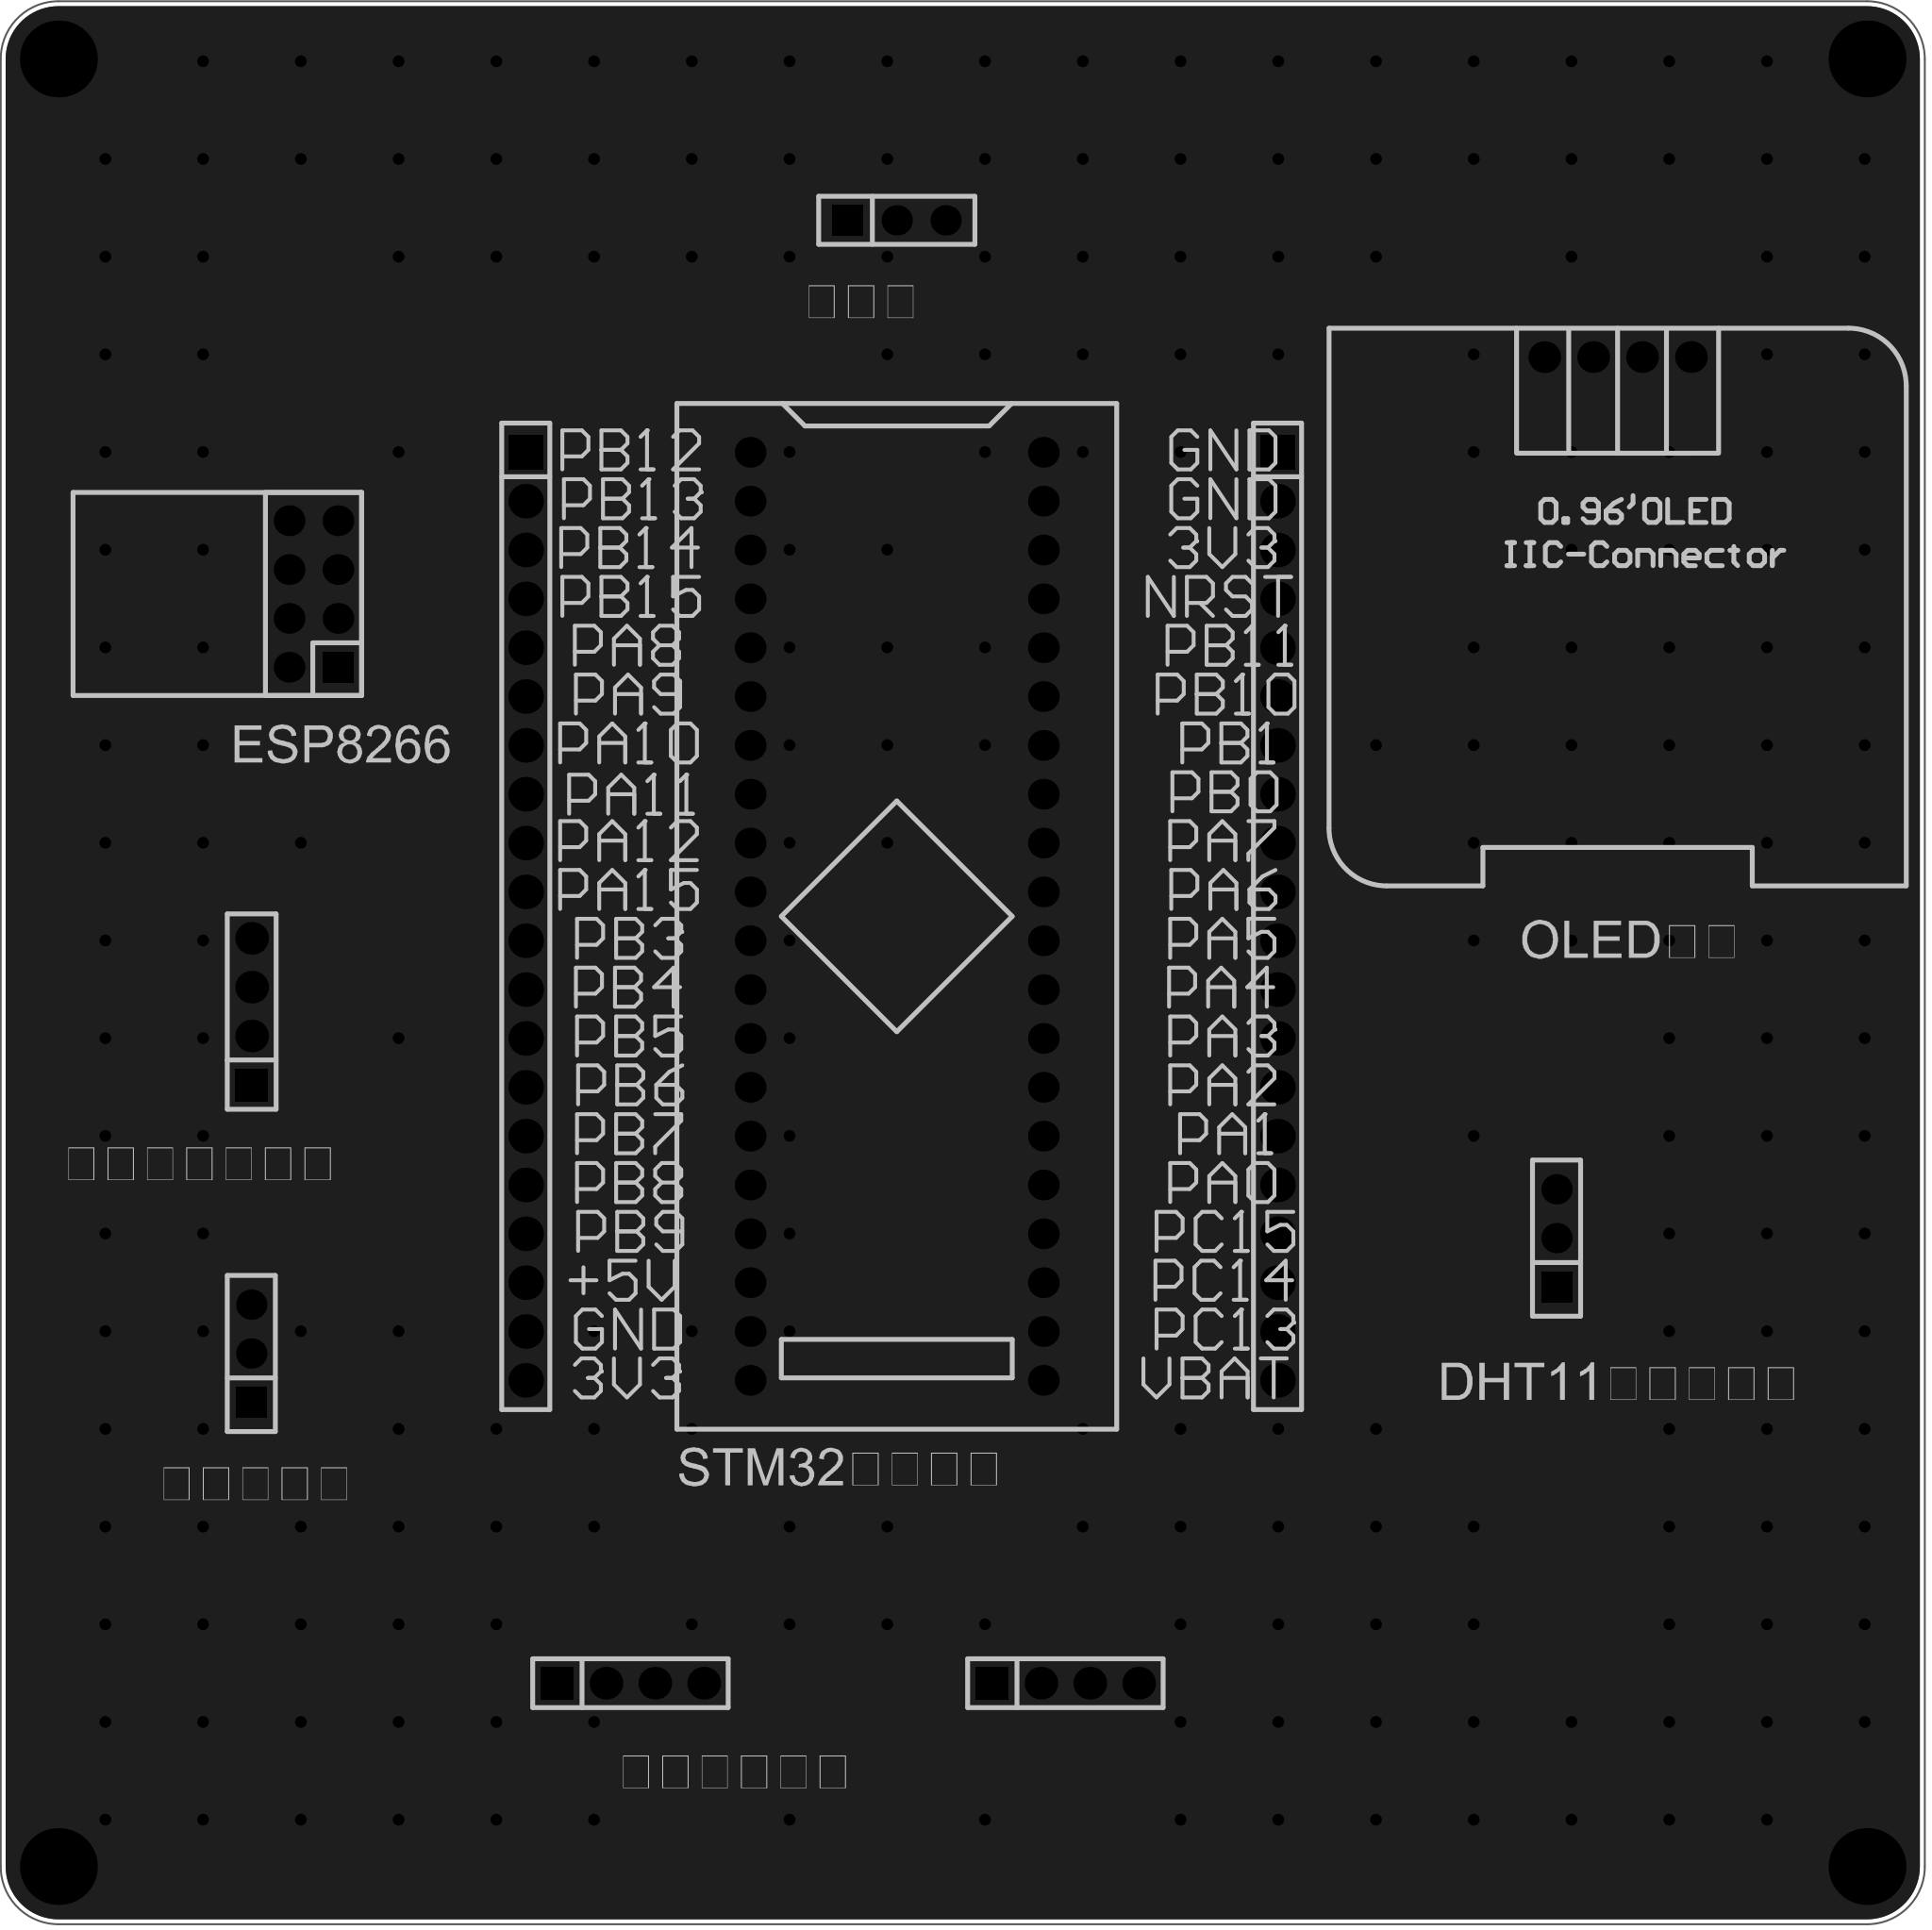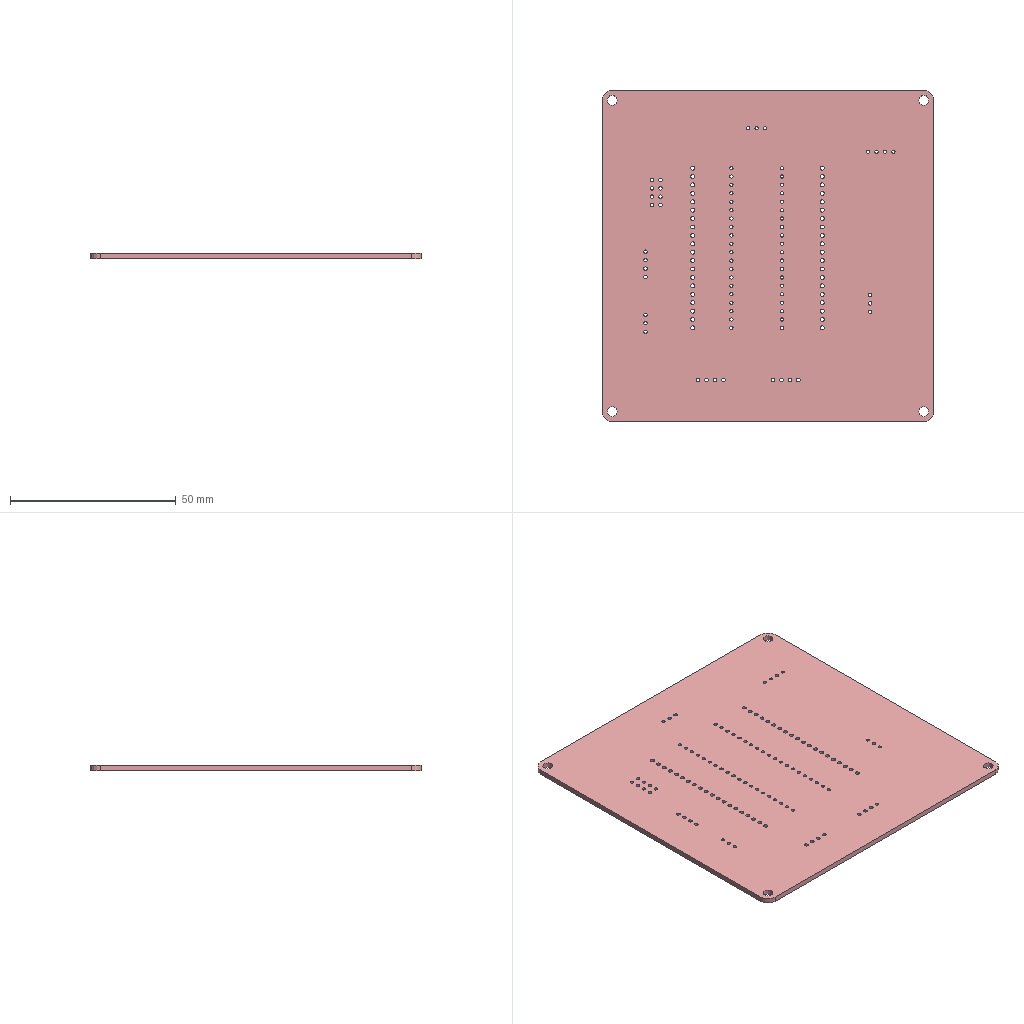Circuit board layout | Altium Designer | box 100 x 100 x 1.6 mm
Layer stack:
# Altium Designer layer stack of  (unit mm; dielectric type: 0 none, 1 core, 2 prepreg, 3 surface material)
index,name,kind,layer,copper_thickness_mm,dielectric_type,dielectric_thickness_mm,dielectric_material,dielectric_constant
0,Top Paste Mask Layer,other,,,,,,
1,Top Silkscreen Layer,other,,,,,,
2,Top Solder Mask Layer,dielectric,,,3,0.01,,3.3
3,Top Layer,copper,Top Layer,0.035,,,,
4,Dielectric1,dielectric,,,3,1.51,FR4,4.5
5,Bottom Layer,copper,Bottom Layer,0.035,,,,
6,Bottom Solder Mask Layer,dielectric,,,3,0.01,,3.3
7,Bottom Silkscreen Layer,other,,,,,,
8,Bottom Paste Mask Layer,other,,,,,,
# drill layer pairs: low layer,high layer
drill_pair,Top Layer,Bottom Layer
Part placement:
Designator,Comment,Layer,Footprint,Center-X(mm),Center-Y(mm),Rotation
U1,STM32F103C8T6-Card,TopLayer,CONN-TH_L53.3-W22.9_STM32F103C8T6-CARD,127.127,131.318,270
H23,HDR2.54-LI-2x4P,TopLayer,HDR-TH_4P-P2.54-V-M,135.89,91.44,0
H24,,TopLayer,HDR-TH_3P-P2.54-V-F,127.127,167.513,0
OLED1,,TopLayer,0.96OLED_4P,164.592,160.401,0
H25,HDR2.54-LI-2x4P,TopLayer,HDR-TH_4P-P2.54-V-M,93.599,126.365,90
H15,,TopLayer,HDR-TH_3P-P2.54-V-F,161.417,114.584,90
H16,,TopLayer,HDR-TH_8P-P2.54-V-F-R2-C4-S2.54-1,96.814,148.082,90
H1,,TopLayer,HDR-TH_20P-P2.54-V-F,107.844,131.318,270
H2,,TopLayer,HDR-TH_20P-P2.54-V-F,146.915,131.318,270
H17,,TopLayer,HDR-TH_3P-P2.54-V-F,93.579,108.585,90
H20,HDR2.54-LI-2x4P,TopLayer,HDR-TH_4P-P2.54-V-M,113.284,91.44,0
Pad and via stacks:
# Altium Designer via and pad stacks of  (unit mm). Each distinct definition once, with the count of objects using it.
# via: kind,start_layer,end_layer,hole_mm,diameter_mm,mode(0 simple;1 top-mid-bottom;2 full stack),diameter_per_layer,count,example_net
# pad: kind,layer,hole_mm,hole_type(0 round;1 square;2 slot),plating,top_size,top_shape(1 round;2 rect;3 octagon;9 rounded rect),mid_size,bottom_size,mode,footprint,size_per_layer,count,example
pad,Multi-Layer,3,0,plated,4x4,1,4x4,4x4,0,,,4,1
pad,Multi-Layer,1,0,plated,1.6x1.6,1,1.6x1.6,1.6x1.6,0,CONN-TH_L53.3-W22.9_STM32F103C8T6-CARD,,40,U1.1
pad,Multi-Layer,1.1,0,plated,1.7x1.7,2,1.7x1.7,1.7x1.7,0,HDR-TH_4P-P2.54-V-M,,3,H23.1
pad,Multi-Layer,1.1,0,plated,1.7x1.7,1,1.7x1.7,1.7x1.7,0,HDR-TH_4P-P2.54-V-M,,9,H23.2
pad,Multi-Layer,1.02,0,plated,1.575x1.575,1,1.575x1.575,1.575x1.575,0,HDR-TH_3P-P2.54-V-F,,6,H24.3
pad,Multi-Layer,1.02,0,plated,1.575x1.575,2,1.575x1.575,1.575x1.575,0,HDR-TH_3P-P2.54-V-F,,3,H24.1
pad,Multi-Layer,1,0,plated,1.65x1.65,1,1.65x1.65,1.65x1.65,0,0.96OLED_4P,,4,OLED1.4
pad,Multi-Layer,1.1,0,plated,1.6x1.6,2,1.6x1.6,1.6x1.6,0,HDR-TH_8P-P2.54-V-F-R2-C4-S2.54-1,,1,H16.1
pad,Multi-Layer,1.1,0,plated,1.6x1.6,1,1.6x1.6,1.6x1.6,0,HDR-TH_8P-P2.54-V-F-R2-C4-S2.54-1,,7,H16.2
pad,Multi-Layer,1.2,0,plated,1.8x1.8,2,1.8x1.8,1.8x1.8,0,HDR-TH_20P-P2.54-V-F,,2,H1.1
pad,Multi-Layer,1.2,0,plated,1.8x1.8,1,1.8x1.8,1.8x1.8,0,HDR-TH_20P-P2.54-V-F,,38,H1.2
via,Top Layer,Bottom Layer,0.3048,0.61,0,,225,GND
Copper pours:
name,layer,net,type(0 solid;1 hatched;2 none)
Bottom Layer-GND,Bottom Layer,GND,0
Top Layer-GND,Top Layer,GND,0